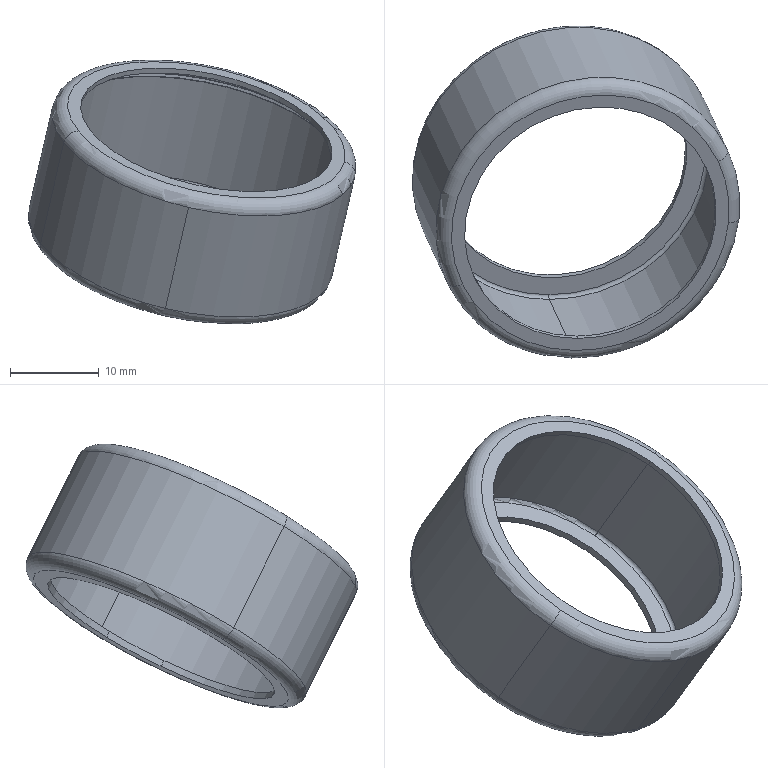Part | SolidWorks | features BaseBody 1 | 1 solid | 40 faces | box 36.983 x 37.484 x 29.782 mm | volume 1472 mm3 | torus 17 | cylinder 15 | plane 4 | cone 3 | spline 1 | commonest cylinder face diameters 28.5 x3 29 x3 33.55 x3 33.75 x3 35.02 x3
STEP:
#1=CARTESIAN_POINT('',(1955.93,-190.672,883.399));
#2=VERTEX_POINT('',#1);
#3=CARTESIAN_POINT('',(1954.896,-184.524,886.692));
#4=VERTEX_POINT('',#3);
#5=CARTESIAN_POINT('',(1942.041,-190.672,886.589));
#6=DIRECTION('',(0.2015,-0.436,0.8771));
#7=DIRECTION('',(-0.9021,-0.4315,-0.007269));
#8=AXIS2_PLACEMENT_3D('',#5,#6,#7);
#9=CIRCLE('',#8,14.25);
#10=EDGE_CURVE('',#2,#4,#9,.T.);
#11=ORIENTED_EDGE('',*,*,#10,.F.);
#12=CARTESIAN_POINT('',(1956.081,-190.999,884.056));
#13=VERTEX_POINT('',#12);
#14=CARTESIAN_POINT('',(1955.918,-190.646,883.346));
#15=DIRECTION('',(0.2015,-0.436,0.8771));
#16=VECTOR('',#15,1000.);
#17=LINE('',#14,#16);
#18=EDGE_CURVE('',#2,#13,#17,.T.);
#19=ORIENTED_EDGE('',*,*,#18,.T.);
#20=CARTESIAN_POINT('',(1955.047,-184.851,887.35));
#21=VERTEX_POINT('',#20);
#22=CARTESIAN_POINT('',(1942.192,-190.999,887.247));
#23=DIRECTION('',(-0.2015,0.436,-0.8771));
#24=DIRECTION('',(0.9021,0.4315,0.007269));
#25=AXIS2_PLACEMENT_3D('',#22,#23,#24);
#26=CIRCLE('',#25,14.25);
#27=EDGE_CURVE('',#21,#13,#26,.T.);
#28=ORIENTED_EDGE('',*,*,#27,.F.);
#29=CARTESIAN_POINT('',(1955.047,-184.851,887.35));
#30=DIRECTION('',(0.2015,-0.436,0.8771));
#31=VECTOR('',#30,1000.);
#32=LINE('',#29,#31);
#33=EDGE_CURVE('',#4,#21,#32,.T.);
#34=ORIENTED_EDGE('',*,*,#33,.F.);
#35=EDGE_LOOP('',(#11,#19,#28,#34));
#36=FACE_OUTER_BOUND('',#35,.T.);
#37=CARTESIAN_POINT('',(1942.029,-190.646,886.536));
#38=DIRECTION('',(0.2015,-0.436,0.8771));
#39=DIRECTION('',(0.9746,0.,-0.2239));
#40=AXIS2_PLACEMENT_3D('',#37,#38,#39);
#41=CYLINDRICAL_SURFACE('',#40,14.25);
#42=ADVANCED_FACE('',(#36),#41,.F.);
#43=CARTESIAN_POINT('',(1957.645,-190.672,883.005));
#44=VERTEX_POINT('',#43);
#45=CARTESIAN_POINT('',(1927.599,-197.58,886.472));
#46=VERTEX_POINT('',#45);
#47=CARTESIAN_POINT('',(1942.041,-190.672,886.589));
#48=DIRECTION('',(-0.2015,0.436,-0.8771));
#49=DIRECTION('',(0.9021,0.4315,0.007269));
#50=AXIS2_PLACEMENT_3D('',#47,#48,#49);
#51=CIRCLE('',#50,16.01);
#52=EDGE_CURVE('',#44,#46,#51,.T.);
#53=ORIENTED_EDGE('',*,*,#52,.F.);
#54=CARTESIAN_POINT('',(1959.409,-191.326,883.984));
#55=VERTEX_POINT('',#54);
#56=CARTESIAN_POINT('',(1957.947,-191.326,884.32));
#57=DIRECTION('',(-0.09761,-0.8999,-0.425));
#58=DIRECTION('',(0.,0.427,-0.9043));
#59=AXIS2_PLACEMENT_3D('',#56,#57,#58);
#60=CIRCLE('',#59,1.5);
#61=EDGE_CURVE('',#44,#55,#60,.T.);
#62=ORIENTED_EDGE('',*,*,#61,.T.);
#63=CARTESIAN_POINT('',(1940.634,-207.084,880.464));
#64=VERTEX_POINT('',#63);
#65=CARTESIAN_POINT('',(1942.344,-191.326,887.904));
#66=DIRECTION('',(-0.2015,0.436,-0.8771));
#67=DIRECTION('',(0.9021,0.4315,0.007269));
#68=AXIS2_PLACEMENT_3D('',#65,#66,#67);
#69=CIRCLE('',#68,17.51);
#70=EDGE_CURVE('',#55,#64,#69,.T.);
#71=ORIENTED_EDGE('',*,*,#70,.T.);
#72=CARTESIAN_POINT('',(1926.548,-198.881,887.777));
#73=VERTEX_POINT('',#72);
#74=CARTESIAN_POINT('',(1942.344,-191.326,887.904));
#75=DIRECTION('',(-0.2015,0.436,-0.8771));
#76=DIRECTION('',(0.9021,0.4315,0.007269));
#77=AXIS2_PLACEMENT_3D('',#74,#75,#76);
#78=CIRCLE('',#77,17.51);
#79=EDGE_CURVE('',#64,#73,#78,.T.);
#80=ORIENTED_EDGE('',*,*,#79,.T.);
#81=CARTESIAN_POINT('',(1927.901,-198.234,887.788));
#82=DIRECTION('',(-0.3816,0.7898,0.4803));
#83=DIRECTION('',(-0.2015,0.436,-0.8771));
#84=AXIS2_PLACEMENT_3D('',#81,#82,#83);
#85=CIRCLE('',#84,1.5);
#86=EDGE_CURVE('',#46,#73,#85,.T.);
#87=ORIENTED_EDGE('',*,*,#86,.F.);
#88=EDGE_LOOP('',(#53,#62,#71,#80,#87));
#89=FACE_OUTER_BOUND('',#88,.T.);
#90=CARTESIAN_POINT('',(1942.344,-191.326,887.904));
#91=DIRECTION('',(0.2015,-0.436,0.8771));
#92=DIRECTION('',(0.9746,0.,-0.2239));
#93=AXIS2_PLACEMENT_3D('',#90,#91,#92);
#94=TOROIDAL_SURFACE('',#93,16.01,1.5);
#95=ADVANCED_FACE('',(#89),#94,.T.);
#96=ORIENTED_EDGE('',*,*,#79,.F.);
#97=CARTESIAN_POINT('',(1943.253,-212.752,891.866));
#98=VERTEX_POINT('',#97);
#99=CARTESIAN_POINT('',(1940.582,-206.971,880.235));
#100=DIRECTION('',(0.2015,-0.436,0.8771));
#101=VECTOR('',#100,1000.);
#102=LINE('',#99,#101);
#103=EDGE_CURVE('',#64,#98,#102,.T.);
#104=ORIENTED_EDGE('',*,*,#103,.T.);
#105=CARTESIAN_POINT('',(1929.167,-204.549,899.179));
#106=VERTEX_POINT('',#105);
#107=CARTESIAN_POINT('',(1944.963,-196.994,899.307));
#108=DIRECTION('',(0.2015,-0.436,0.8771));
#109=DIRECTION('',(0.9726,0.195,-0.1265));
#110=AXIS2_PLACEMENT_3D('',#107,#108,#109);
#111=CIRCLE('',#110,17.51);
#112=EDGE_CURVE('',#106,#98,#111,.T.);
#113=ORIENTED_EDGE('',*,*,#112,.F.);
#114=CARTESIAN_POINT('',(1926.548,-198.881,887.777));
#115=DIRECTION('',(-0.2015,0.436,-0.8771));
#116=VECTOR('',#115,1000.);
#117=LINE('',#114,#116);
#118=EDGE_CURVE('',#106,#73,#117,.T.);
#119=ORIENTED_EDGE('',*,*,#118,.T.);
#120=EDGE_LOOP('',(#96,#104,#113,#119));
#121=FACE_OUTER_BOUND('',#120,.T.);
#122=CARTESIAN_POINT('',(1942.291,-191.213,887.676));
#123=DIRECTION('',(0.2015,-0.436,0.8771));
#124=DIRECTION('',(-0.09761,-0.8999,-0.425));
#125=AXIS2_PLACEMENT_3D('',#122,#123,#124);
#126=CYLINDRICAL_SURFACE('',#125,17.51);
#127=ADVANCED_FACE('',(#121),#126,.T.);
#128=ORIENTED_EDGE('',*,*,#112,.T.);
#129=CARTESIAN_POINT('',(1962.028,-196.994,895.387));
#130=VERTEX_POINT('',#129);
#131=CARTESIAN_POINT('',(1944.963,-196.994,899.307));
#132=DIRECTION('',(0.2015,-0.436,0.8771));
#133=DIRECTION('',(0.9726,0.195,-0.1265));
#134=AXIS2_PLACEMENT_3D('',#131,#132,#133);
#135=CIRCLE('',#134,17.51);
#136=EDGE_CURVE('',#98,#130,#135,.T.);
#137=ORIENTED_EDGE('',*,*,#136,.T.);
#138=CARTESIAN_POINT('',(1960.868,-197.648,897.038));
#139=VERTEX_POINT('',#138);
#140=CARTESIAN_POINT('',(1960.566,-196.994,895.723));
#141=DIRECTION('',(-0.09761,-0.8999,-0.425));
#142=DIRECTION('',(0.,0.427,-0.9043));
#143=AXIS2_PLACEMENT_3D('',#140,#141,#142);
#144=CIRCLE('',#143,1.5);
#145=EDGE_CURVE('',#130,#139,#144,.T.);
#146=ORIENTED_EDGE('',*,*,#145,.T.);
#147=CARTESIAN_POINT('',(1930.822,-204.556,900.506));
#148=VERTEX_POINT('',#147);
#149=CARTESIAN_POINT('',(1945.265,-197.648,900.622));
#150=DIRECTION('',(-0.2015,0.436,-0.8771));
#151=DIRECTION('',(0.9021,0.4315,0.007269));
#152=AXIS2_PLACEMENT_3D('',#149,#150,#151);
#153=CIRCLE('',#152,16.01);
#154=EDGE_CURVE('',#139,#148,#153,.T.);
#155=ORIENTED_EDGE('',*,*,#154,.T.);
#156=CARTESIAN_POINT('',(1930.52,-203.902,899.19));
#157=DIRECTION('',(0.3816,-0.7898,-0.4803));
#158=DIRECTION('',(-0.9021,-0.4315,-0.007269));
#159=AXIS2_PLACEMENT_3D('',#156,#157,#158);
#160=CIRCLE('',#159,1.5);
#161=EDGE_CURVE('',#148,#106,#160,.T.);
#162=ORIENTED_EDGE('',*,*,#161,.T.);
#163=EDGE_LOOP('',(#128,#137,#146,#155,#162));
#164=FACE_OUTER_BOUND('',#163,.T.);
#165=CARTESIAN_POINT('',(1944.963,-196.994,899.307));
#166=DIRECTION('',(0.2015,-0.436,0.8771));
#167=DIRECTION('',(0.9746,0.,-0.2239));
#168=AXIS2_PLACEMENT_3D('',#165,#166,#167);
#169=TOROIDAL_SURFACE('',#168,16.01,1.5);
#170=ADVANCED_FACE('',(#164),#169,.T.);
#171=CARTESIAN_POINT('',(1943.729,-210.436,893.934));
#172=VERTEX_POINT('',#171);
#173=CARTESIAN_POINT('',(1958.224,-191.131,900.201));
#174=VERTEX_POINT('',#173);
#175=CARTESIAN_POINT('',(1945.144,-197.387,900.096));
#176=DIRECTION('',(0.2015,-0.436,0.8771));
#177=DIRECTION('',(-0.9021,-0.4315,-0.007269));
#178=AXIS2_PLACEMENT_3D('',#175,#176,#177);
#179=CIRCLE('',#178,14.5);
#180=EDGE_CURVE('',#172,#174,#179,.T.);
#181=ORIENTED_EDGE('',*,*,#180,.F.);
#182=CARTESIAN_POINT('',(1943.849,-210.697,894.461));
#183=VERTEX_POINT('',#182);
#184=CARTESIAN_POINT('',(1943.716,-210.41,893.882));
#185=DIRECTION('',(0.2015,-0.436,0.8771));
#186=VECTOR('',#185,1000.);
#187=LINE('',#184,#186);
#188=EDGE_CURVE('',#172,#183,#187,.T.);
#189=ORIENTED_EDGE('',*,*,#188,.T.);
#190=CARTESIAN_POINT('',(1958.345,-191.392,900.728));
#191=VERTEX_POINT('',#190);
#192=CARTESIAN_POINT('',(1945.265,-197.648,900.622));
#193=DIRECTION('',(-0.2015,0.436,-0.8771));
#194=DIRECTION('',(0.9021,0.4315,0.007269));
#195=AXIS2_PLACEMENT_3D('',#192,#193,#194);
#196=CIRCLE('',#195,14.5);
#197=EDGE_CURVE('',#191,#183,#196,.T.);
#198=ORIENTED_EDGE('',*,*,#197,.F.);
#199=CARTESIAN_POINT('',(1958.345,-191.392,900.728));
#200=DIRECTION('',(0.2015,-0.436,0.8771));
#201=VECTOR('',#200,1000.);
#202=LINE('',#199,#201);
#203=EDGE_CURVE('',#174,#191,#202,.T.);
#204=ORIENTED_EDGE('',*,*,#203,.F.);
#205=EDGE_LOOP('',(#181,#189,#198,#204));
#206=FACE_OUTER_BOUND('',#205,.T.);
#207=CARTESIAN_POINT('',(1945.132,-197.36,900.043));
#208=DIRECTION('',(0.2015,-0.436,0.8771));
#209=DIRECTION('',(-0.09761,-0.8999,-0.425));
#210=AXIS2_PLACEMENT_3D('',#207,#208,#209);
#211=CYLINDRICAL_SURFACE('',#210,14.5);
#212=ADVANCED_FACE('',(#206),#211,.F.);
#213=CARTESIAN_POINT('',(1960.286,-189.931,899.868));
#214=VERTEX_POINT('',#213);
#215=CARTESIAN_POINT('',(1943.416,-212.399,892.574));
#216=VERTEX_POINT('',#215);
#217=CARTESIAN_POINT('',(1945.063,-197.212,899.745));
#218=DIRECTION('',(-0.2015,0.436,-0.8771));
#219=DIRECTION('',(0.9021,0.4315,0.007269));
#220=AXIS2_PLACEMENT_3D('',#217,#218,#219);
#221=CIRCLE('',#220,16.875);
#222=EDGE_CURVE('',#214,#216,#221,.T.);
#223=ORIENTED_EDGE('',*,*,#222,.T.);
#224=CARTESIAN_POINT('',(1943.536,-212.213,893.095));
#225=VERTEX_POINT('',#224);
#226=CARTESIAN_POINT('',(1943.455,-212.039,892.744));
#227=DIRECTION('',(-0.9746,0.,0.2239));
#228=DIRECTION('',(0.2239,0.,0.9746));
#229=AXIS2_PLACEMENT_3D('',#226,#227,#228);
#230=CIRCLE('',#229,0.4);
#231=EDGE_CURVE('',#216,#225,#230,.T.);
#232=ORIENTED_EDGE('',*,*,#231,.T.);
#233=CARTESIAN_POINT('',(1960.006,-190.278,900.216));
#234=VERTEX_POINT('',#233);
#235=CARTESIAN_POINT('',(1945.144,-197.387,900.096));
#236=DIRECTION('',(-0.2015,0.436,-0.8771));
#237=DIRECTION('',(0.9021,0.4315,0.007269));
#238=AXIS2_PLACEMENT_3D('',#235,#236,#237);
#239=CIRCLE('',#238,16.475);
#240=EDGE_CURVE('',#234,#225,#239,.T.);
#241=ORIENTED_EDGE('',*,*,#240,.F.);
#242=CARTESIAN_POINT('',(1959.926,-190.104,899.865));
#243=DIRECTION('',(-0.3816,0.7898,0.4803));
#244=DIRECTION('',(0.2015,-0.436,0.8771));
#245=AXIS2_PLACEMENT_3D('',#242,#243,#244);
#246=CIRCLE('',#245,0.4);
#247=EDGE_CURVE('',#234,#214,#246,.T.);
#248=ORIENTED_EDGE('',*,*,#247,.T.);
#249=EDGE_LOOP('',(#223,#232,#241,#248));
#250=FACE_OUTER_BOUND('',#249,.T.);
#251=CARTESIAN_POINT('',(1945.063,-197.212,899.745));
#252=DIRECTION('',(0.2015,-0.436,0.8771));
#253=DIRECTION('',(-0.09761,-0.8999,-0.425));
#254=AXIS2_PLACEMENT_3D('',#251,#252,#253);
#255=TOROIDAL_SURFACE('',#254,16.475,0.4);
#256=ADVANCED_FACE('',(#250),#255,.F.);
#257=CARTESIAN_POINT('',(1943.235,-212.006,891.784));
#258=VERTEX_POINT('',#257);
#259=CARTESIAN_POINT('',(1960.105,-189.539,899.078));
#260=VERTEX_POINT('',#259);
#261=CARTESIAN_POINT('',(1944.882,-196.82,898.955));
#262=DIRECTION('',(0.2015,-0.436,0.8771));
#263=DIRECTION('',(-0.9021,-0.4315,-0.007269));
#264=AXIS2_PLACEMENT_3D('',#261,#262,#263);
#265=CIRCLE('',#264,16.875);
#266=EDGE_CURVE('',#258,#260,#265,.T.);
#267=ORIENTED_EDGE('',*,*,#266,.F.);
#268=CARTESIAN_POINT('',(1943.223,-211.98,891.732));
#269=DIRECTION('',(0.2015,-0.436,0.8771));
#270=VECTOR('',#269,1000.);
#271=LINE('',#268,#270);
#272=EDGE_CURVE('',#258,#216,#271,.T.);
#273=ORIENTED_EDGE('',*,*,#272,.T.);
#274=ORIENTED_EDGE('',*,*,#222,.F.);
#275=CARTESIAN_POINT('',(1960.286,-189.931,899.868));
#276=DIRECTION('',(0.2015,-0.436,0.8771));
#277=VECTOR('',#276,1000.);
#278=LINE('',#275,#277);
#279=EDGE_CURVE('',#260,#214,#278,.T.);
#280=ORIENTED_EDGE('',*,*,#279,.F.);
#281=EDGE_LOOP('',(#267,#273,#274,#280));
#282=FACE_OUTER_BOUND('',#281,.T.);
#283=CARTESIAN_POINT('',(1944.87,-196.793,898.903));
#284=DIRECTION('',(0.2015,-0.436,0.8771));
#285=DIRECTION('',(-0.09761,-0.8999,-0.425));
#286=AXIS2_PLACEMENT_3D('',#283,#284,#285);
#287=CYLINDRICAL_SURFACE('',#286,16.875);
#288=ADVANCED_FACE('',(#282),#287,.F.);
#289=CARTESIAN_POINT('',(1960.088,-189.519,899.033));
#290=VERTEX_POINT('',#289);
#291=CARTESIAN_POINT('',(1943.225,-211.977,891.742));
#292=VERTEX_POINT('',#291);
#293=CARTESIAN_POINT('',(1944.871,-196.797,898.91));
#294=DIRECTION('',(-0.2015,0.436,-0.8771));
#295=DIRECTION('',(0.9021,0.4315,0.007269));
#296=AXIS2_PLACEMENT_3D('',#293,#294,#295);
#297=CIRCLE('',#296,16.868);
#298=EDGE_CURVE('',#290,#292,#297,.T.);
#299=ORIENTED_EDGE('',*,*,#298,.T.);
#300=CARTESIAN_POINT('',(1943.254,-211.826,891.869));
#301=DIRECTION('',(-0.9746,0.,0.2239));
#302=DIRECTION('',(0.2239,0.,0.9746));
#303=AXIS2_PLACEMENT_3D('',#300,#301,#302);
#304=CIRCLE('',#303,0.2);
#305=EDGE_CURVE('',#292,#258,#304,.T.);
#306=ORIENTED_EDGE('',*,*,#305,.T.);
#307=ORIENTED_EDGE('',*,*,#266,.T.);
#308=CARTESIAN_POINT('',(1959.925,-189.625,899.077));
#309=DIRECTION('',(-0.3816,0.7898,0.4803));
#310=DIRECTION('',(0.9021,0.4315,0.007269));
#311=AXIS2_PLACEMENT_3D('',#308,#309,#310);
#312=CIRCLE('',#311,0.2);
#313=EDGE_CURVE('',#260,#290,#312,.T.);
#314=ORIENTED_EDGE('',*,*,#313,.T.);
#315=EDGE_LOOP('',(#299,#306,#307,#314));
#316=FACE_OUTER_BOUND('',#315,.T.);
#317=CARTESIAN_POINT('',(1944.882,-196.82,898.955));
#318=DIRECTION('',(0.2015,-0.436,0.8771));
#319=DIRECTION('',(-0.09761,-0.8999,-0.425));
#320=AXIS2_PLACEMENT_3D('',#317,#318,#319);
#321=TOROIDAL_SURFACE('',#320,16.675,0.2);
#322=ADVANCED_FACE('',(#316),#321,.F.);
#323=CARTESIAN_POINT('',(1943.168,-211.759,891.496));
#324=VERTEX_POINT('',#323);
#325=CARTESIAN_POINT('',(1959.946,-189.416,898.749));
#326=VERTEX_POINT('',#325);
#327=CARTESIAN_POINT('',(1944.807,-196.656,898.627));
#328=DIRECTION('',(0.2015,-0.436,0.8771));
#329=DIRECTION('',(-0.9021,-0.4315,-0.007269));
#330=AXIS2_PLACEMENT_3D('',#327,#328,#329);
#331=CIRCLE('',#330,16.782);
#332=EDGE_CURVE('',#324,#326,#331,.T.);
#333=ORIENTED_EDGE('',*,*,#332,.F.);
#334=CARTESIAN_POINT('',(1943.158,-211.72,891.452));
#335=DIRECTION('',(0.1693,-0.6541,0.7372));
#336=VECTOR('',#335,1000.);
#337=LINE('',#334,#336);
#338=EDGE_CURVE('',#324,#292,#337,.T.);
#339=ORIENTED_EDGE('',*,*,#338,.T.);
#340=ORIENTED_EDGE('',*,*,#298,.F.);
#341=CARTESIAN_POINT('',(1960.088,-189.519,899.033));
#342=DIRECTION('',(0.4281,-0.3095,0.8491));
#343=VECTOR('',#342,1000.);
#344=LINE('',#341,#343);
#345=EDGE_CURVE('',#326,#290,#344,.T.);
#346=ORIENTED_EDGE('',*,*,#345,.F.);
#347=EDGE_LOOP('',(#333,#339,#340,#346));
#348=FACE_OUTER_BOUND('',#347,.T.);
#349=CARTESIAN_POINT('',(1944.795,-196.631,898.576));
#350=DIRECTION('',(0.2015,-0.436,0.8771));
#351=DIRECTION('',(-0.09761,-0.8999,-0.425));
#352=AXIS2_PLACEMENT_3D('',#349,#350,#351);
#353=CONICAL_SURFACE('',#352,16.766,0.2618);
#354=ADVANCED_FACE('',(#348),#353,.F.);
#355=CARTESIAN_POINT('',(1929.668,-203.897,898.505));
#356=VERTEX_POINT('',#355);
#357=CARTESIAN_POINT('',(1944.807,-196.656,898.627));
#358=DIRECTION('',(0.2015,-0.436,0.8771));
#359=DIRECTION('',(-0.9021,-0.4315,-0.007269));
#360=AXIS2_PLACEMENT_3D('',#357,#358,#359);
#361=CIRCLE('',#360,16.782);
#362=EDGE_CURVE('',#356,#324,#361,.T.);
#363=ORIENTED_EDGE('',*,*,#362,.T.);
#364=CARTESIAN_POINT('',(1943.159,-211.73,891.453));
#365=VERTEX_POINT('',#364);
#366=CARTESIAN_POINT('',(1943.139,-211.91,891.368));
#367=DIRECTION('',(-0.9746,0.,0.2239));
#368=DIRECTION('',(0.2239,0.,0.9746));
#369=AXIS2_PLACEMENT_3D('',#366,#367,#368);
#370=CIRCLE('',#369,0.2);
#371=EDGE_CURVE('',#324,#365,#370,.T.);
#372=ORIENTED_EDGE('',*,*,#371,.T.);
#373=CARTESIAN_POINT('',(1929.663,-203.872,898.46));
#374=VERTEX_POINT('',#373);
#375=CARTESIAN_POINT('',(1944.796,-196.634,898.582));
#376=DIRECTION('',(-0.2015,0.436,-0.8771));
#377=DIRECTION('',(0.9021,0.4315,0.007269));
#378=AXIS2_PLACEMENT_3D('',#375,#376,#377);
#379=CIRCLE('',#378,16.775);
#380=EDGE_CURVE('',#365,#374,#379,.T.);
#381=ORIENTED_EDGE('',*,*,#380,.T.);
#382=CARTESIAN_POINT('',(1929.483,-203.958,898.458));
#383=DIRECTION('',(0.3816,-0.7898,-0.4803));
#384=DIRECTION('',(0.9235,0.3039,0.234));
#385=AXIS2_PLACEMENT_3D('',#382,#383,#384);
#386=CIRCLE('',#385,0.2);
#387=EDGE_CURVE('',#374,#356,#386,.T.);
#388=ORIENTED_EDGE('',*,*,#387,.T.);
#389=EDGE_LOOP('',(#363,#372,#381,#388));
#390=FACE_OUTER_BOUND('',#389,.T.);
#391=CARTESIAN_POINT('',(1944.796,-196.634,898.582));
#392=DIRECTION('',(0.2015,-0.436,0.8771));
#393=DIRECTION('',(-0.09761,-0.8999,-0.425));
#394=AXIS2_PLACEMENT_3D('',#391,#392,#393);
#395=TOROIDAL_SURFACE('',#394,16.975,0.2);
#396=ADVANCED_FACE('',(#390),#395,.T.);
#397=CARTESIAN_POINT('',(1940.636,-206.27,880.469));
#398=VERTEX_POINT('',#397);
#399=CARTESIAN_POINT('',(1957.406,-183.936,887.719));
#400=VERTEX_POINT('',#399);
#401=CARTESIAN_POINT('',(1942.273,-191.173,887.597));
#402=DIRECTION('',(0.2015,-0.436,0.8771));
#403=DIRECTION('',(-0.9021,-0.4315,-0.007269));
#404=AXIS2_PLACEMENT_3D('',#401,#402,#403);
#405=CIRCLE('',#404,16.775);
#406=EDGE_CURVE('',#398,#400,#405,.T.);
#407=ORIENTED_EDGE('',*,*,#406,.F.);
#408=CARTESIAN_POINT('',(1940.585,-206.161,880.249));
#409=DIRECTION('',(0.2015,-0.436,0.8771));
#410=VECTOR('',#409,1000.);
#411=LINE('',#408,#410);
#412=EDGE_CURVE('',#398,#365,#411,.T.);
#413=ORIENTED_EDGE('',*,*,#412,.T.);
#414=CARTESIAN_POINT('',(1959.929,-189.396,898.704));
#415=VERTEX_POINT('',#414);
#416=CARTESIAN_POINT('',(1944.796,-196.634,898.582));
#417=DIRECTION('',(-0.2015,0.436,-0.8771));
#418=DIRECTION('',(0.9021,0.4315,0.007269));
#419=AXIS2_PLACEMENT_3D('',#416,#417,#418);
#420=CIRCLE('',#419,16.775);
#421=EDGE_CURVE('',#415,#365,#420,.T.);
#422=ORIENTED_EDGE('',*,*,#421,.F.);
#423=CARTESIAN_POINT('',(1959.929,-189.396,898.704));
#424=DIRECTION('',(-0.2015,0.436,-0.8771));
#425=VECTOR('',#424,1000.);
#426=LINE('',#423,#425);
#427=EDGE_CURVE('',#415,#400,#426,.T.);
#428=ORIENTED_EDGE('',*,*,#427,.T.);
#429=EDGE_LOOP('',(#407,#413,#422,#428));
#430=FACE_OUTER_BOUND('',#429,.T.);
#431=CARTESIAN_POINT('',(1942.223,-191.064,887.378));
#432=DIRECTION('',(0.2015,-0.436,0.8771));
#433=DIRECTION('',(-0.09761,-0.8999,-0.425));
#434=AXIS2_PLACEMENT_3D('',#431,#432,#433);
#435=CYLINDRICAL_SURFACE('',#434,16.775);
#436=ADVANCED_FACE('',(#430),#435,.F.);
#437=CARTESIAN_POINT('',(1940.594,-205.735,880.288));
#438=VERTEX_POINT('',#437);
#439=CARTESIAN_POINT('',(1956.964,-183.934,887.366));
#440=VERTEX_POINT('',#439);
#441=CARTESIAN_POINT('',(1942.192,-190.999,887.247));
#442=DIRECTION('',(0.2015,-0.436,0.8771));
#443=DIRECTION('',(-0.9021,-0.4315,-0.007269));
#444=AXIS2_PLACEMENT_3D('',#441,#442,#443);
#445=CIRCLE('',#444,16.375);
#446=EDGE_CURVE('',#438,#440,#445,.T.);
#447=ORIENTED_EDGE('',*,*,#446,.F.);
#448=CARTESIAN_POINT('',(1940.675,-205.91,880.639));
#449=DIRECTION('',(-0.9746,0.,0.2239));
#450=DIRECTION('',(0.2239,0.,0.9746));
#451=AXIS2_PLACEMENT_3D('',#448,#449,#450);
#452=CIRCLE('',#451,0.4);
#453=EDGE_CURVE('',#438,#398,#452,.T.);
#454=ORIENTED_EDGE('',*,*,#453,.T.);
#455=ORIENTED_EDGE('',*,*,#406,.T.);
#456=CARTESIAN_POINT('',(1957.045,-184.108,887.716));
#457=DIRECTION('',(-0.3816,0.7898,0.4803));
#458=DIRECTION('',(0.9021,0.4315,0.007269));
#459=AXIS2_PLACEMENT_3D('',#456,#457,#458);
#460=CIRCLE('',#459,0.4);
#461=EDGE_CURVE('',#400,#440,#460,.T.);
#462=ORIENTED_EDGE('',*,*,#461,.T.);
#463=EDGE_LOOP('',(#447,#454,#455,#462));
#464=FACE_OUTER_BOUND('',#463,.T.);
#465=CARTESIAN_POINT('',(1942.273,-191.173,887.597));
#466=DIRECTION('',(0.2015,-0.436,0.8771));
#467=DIRECTION('',(-0.09761,-0.8999,-0.425));
#468=AXIS2_PLACEMENT_3D('',#465,#466,#467);
#469=TOROIDAL_SURFACE('',#468,16.375,0.4);
#470=ADVANCED_FACE('',(#464),#469,.F.);
#471=ORIENTED_EDGE('',*,*,#345,.T.);
#472=CARTESIAN_POINT('',(1929.655,-204.075,898.787));
#473=VERTEX_POINT('',#472);
#474=CARTESIAN_POINT('',(1944.871,-196.797,898.91));
#475=DIRECTION('',(-0.2015,0.436,-0.8771));
#476=DIRECTION('',(-0.9021,-0.4315,-0.007269));
#477=AXIS2_PLACEMENT_3D('',#474,#475,#476);
#478=CIRCLE('',#477,16.868);
#479=EDGE_CURVE('',#473,#290,#478,.T.);
#480=ORIENTED_EDGE('',*,*,#479,.F.);
#481=CARTESIAN_POINT('',(1929.655,-204.075,898.787));
#482=DIRECTION('',(0.03888,0.5328,-0.8453));
#483=VECTOR('',#482,1000.);
#484=LINE('',#481,#483);
#485=EDGE_CURVE('',#473,#356,#484,.T.);
#486=ORIENTED_EDGE('',*,*,#485,.T.);
#487=CARTESIAN_POINT('',(1944.807,-196.656,898.627));
#488=DIRECTION('',(0.2015,-0.436,0.8771));
#489=DIRECTION('',(0.9021,0.4315,0.007269));
#490=AXIS2_PLACEMENT_3D('',#487,#488,#489);
#491=CIRCLE('',#490,16.782);
#492=EDGE_CURVE('',#326,#356,#491,.T.);
#493=ORIENTED_EDGE('',*,*,#492,.F.);
#494=EDGE_LOOP('',(#471,#480,#486,#493));
#495=FACE_OUTER_BOUND('',#494,.T.);
#496=CARTESIAN_POINT('',(1944.795,-196.631,898.576));
#497=DIRECTION('',(0.2015,-0.436,0.8771));
#498=DIRECTION('',(-0.09761,-0.8999,-0.425));
#499=AXIS2_PLACEMENT_3D('',#496,#497,#498);
#500=CONICAL_SURFACE('',#499,16.766,0.2618);
#501=ADVANCED_FACE('',(#495),#500,.F.);
#502=CARTESIAN_POINT('',(1960.109,-189.31,898.705));
#503=DIRECTION('',(0.3816,-0.7898,-0.4803));
#504=DIRECTION('',(-0.8192,-0.5296,0.22));
#505=AXIS2_PLACEMENT_3D('',#502,#503,#504);
#506=CIRCLE('',#505,0.2);
#507=EDGE_CURVE('',#326,#415,#506,.T.);
#508=ORIENTED_EDGE('',*,*,#507,.F.);
#509=ORIENTED_EDGE('',*,*,#492,.T.);
#510=ORIENTED_EDGE('',*,*,#387,.F.);
#511=CARTESIAN_POINT('',(1944.796,-196.634,898.582));
#512=DIRECTION('',(-0.2015,0.436,-0.8771));
#513=DIRECTION('',(-0.9021,-0.4315,-0.007269));
#514=AXIS2_PLACEMENT_3D('',#511,#512,#513);
#515=CIRCLE('',#514,16.775);
#516=EDGE_CURVE('',#374,#415,#515,.T.);
#517=ORIENTED_EDGE('',*,*,#516,.T.);
#518=EDGE_LOOP('',(#508,#509,#510,#517));
#519=FACE_OUTER_BOUND('',#518,.T.);
#520=CARTESIAN_POINT('',(1944.796,-196.634,898.582));
#521=DIRECTION('',(0.2015,-0.436,0.8771));
#522=DIRECTION('',(-0.09761,-0.8999,-0.425));
#523=AXIS2_PLACEMENT_3D('',#520,#521,#522);
#524=TOROIDAL_SURFACE('',#523,16.975,0.2);
#525=ADVANCED_FACE('',(#519),#524,.T.);
#526=ORIENTED_EDGE('',*,*,#427,.F.);
#527=ORIENTED_EDGE('',*,*,#516,.F.);
#528=CARTESIAN_POINT('',(1927.14,-198.411,887.475));
#529=VERTEX_POINT('',#528);
#530=CARTESIAN_POINT('',(1929.663,-203.872,898.46));
#531=DIRECTION('',(0.2015,-0.436,0.8771));
#532=VECTOR('',#531,1000.);
#533=LINE('',#530,#532);
#534=EDGE_CURVE('',#529,#374,#533,.T.);
#535=ORIENTED_EDGE('',*,*,#534,.F.);
#536=CARTESIAN_POINT('',(1942.273,-191.173,887.597));
#537=DIRECTION('',(0.2015,-0.436,0.8771));
#538=DIRECTION('',(0.9021,0.4315,0.007269));
#539=AXIS2_PLACEMENT_3D('',#536,#537,#538);
#540=CIRCLE('',#539,16.775);
#541=EDGE_CURVE('',#400,#529,#540,.T.);
#542=ORIENTED_EDGE('',*,*,#541,.F.);
#543=EDGE_LOOP('',(#526,#527,#535,#542));
#544=FACE_OUTER_BOUND('',#543,.T.);
#545=CARTESIAN_POINT('',(1942.223,-191.064,887.378));
#546=DIRECTION('',(0.2015,-0.436,0.8771));
#547=DIRECTION('',(-0.09761,-0.8999,-0.425));
#548=AXIS2_PLACEMENT_3D('',#545,#546,#547);
#549=CYLINDRICAL_SURFACE('',#548,16.775);
#550=ADVANCED_FACE('',(#544),#549,.F.);
#551=ORIENTED_EDGE('',*,*,#461,.F.);
#552=ORIENTED_EDGE('',*,*,#541,.T.);
#553=CARTESIAN_POINT('',(1927.42,-198.064,887.128));
#554=VERTEX_POINT('',#553);
#555=CARTESIAN_POINT('',(1927.501,-198.238,887.478));
#556=DIRECTION('',(-0.3816,0.7898,0.4803));
#557=DIRECTION('',(-0.9021,-0.4315,-0.007269));
#558=AXIS2_PLACEMENT_3D('',#555,#556,#557);
#559=CIRCLE('',#558,0.4);
#560=EDGE_CURVE('',#554,#529,#559,.T.);
#561=ORIENTED_EDGE('',*,*,#560,.F.);
#562=CARTESIAN_POINT('',(1942.192,-190.999,887.247));
#563=DIRECTION('',(0.2015,-0.436,0.8771));
#564=DIRECTION('',(0.9021,0.4315,0.007269));
#565=AXIS2_PLACEMENT_3D('',#562,#563,#564);
#566=CIRCLE('',#565,16.375);
#567=EDGE_CURVE('',#440,#554,#566,.T.);
#568=ORIENTED_EDGE('',*,*,#567,.F.);
#569=EDGE_LOOP('',(#551,#552,#561,#568));
#570=FACE_OUTER_BOUND('',#569,.T.);
#571=CARTESIAN_POINT('',(1942.273,-191.173,887.597));
#572=DIRECTION('',(0.2015,-0.436,0.8771));
#573=DIRECTION('',(-0.09761,-0.8999,-0.425));
#574=AXIS2_PLACEMENT_3D('',#571,#572,#573);
#575=TOROIDAL_SURFACE('',#574,16.375,0.4);
#576=ADVANCED_FACE('',(#570),#575,.F.);
#577=CARTESIAN_POINT('',(1942.192,-190.999,887.247));
#578=DIRECTION('',(0.2015,-0.436,0.8771));
#579=DIRECTION('',(-0.9021,-0.4315,-0.007269));
#580=AXIS2_PLACEMENT_3D('',#577,#578,#579);
#581=CIRCLE('',#580,16.375);
#582=EDGE_CURVE('',#554,#438,#581,.T.);
#583=ORIENTED_EDGE('',*,*,#582,.T.);
#584=ORIENTED_EDGE('',*,*,#446,.T.);
#585=ORIENTED_EDGE('',*,*,#567,.T.);
#586=EDGE_LOOP('',(#583,#584,#585));
#587=FACE_OUTER_BOUND('',#586,.T.);
#588=ORIENTED_EDGE('',*,*,#27,.T.);
#589=CARTESIAN_POINT('',(1929.337,-197.147,887.143));
#590=VERTEX_POINT('',#589);
#591=CARTESIAN_POINT('',(1942.192,-190.999,887.247));
#592=DIRECTION('',(-0.2015,0.436,-0.8771));
#593=DIRECTION('',(0.9021,0.4315,0.007269));
#594=AXIS2_PLACEMENT_3D('',#591,#592,#593);
#595=CIRCLE('',#594,14.25);
#596=EDGE_CURVE('',#13,#590,#595,.T.);
#597=ORIENTED_EDGE('',*,*,#596,.T.);
#598=CARTESIAN_POINT('',(1942.192,-190.999,887.247));
#599=DIRECTION('',(-0.2015,0.436,-0.8771));
#600=DIRECTION('',(-0.9021,-0.4315,-0.007269));
#601=AXIS2_PLACEMENT_3D('',#598,#599,#600);
#602=CIRCLE('',#601,14.25);
#603=EDGE_CURVE('',#590,#21,#602,.T.);
#604=ORIENTED_EDGE('',*,*,#603,.T.);
#605=EDGE_LOOP('',(#588,#597,#604));
#606=FACE_BOUND('',#605,.T.);
#607=CARTESIAN_POINT('',(1957.134,-206.325,876.196));
#608=DIRECTION('',(0.2015,-0.436,0.8771));
#609=DIRECTION('',(0.09761,0.8999,0.425));
#610=AXIS2_PLACEMENT_3D('',#607,#608,#609);
#611=PLANE('',#610);
#612=ADVANCED_FACE('',(#587,#606),#611,.T.);
#613=ORIENTED_EDGE('',*,*,#453,.F.);
#614=ORIENTED_EDGE('',*,*,#582,.F.);
#615=ORIENTED_EDGE('',*,*,#560,.T.);
#616=CARTESIAN_POINT('',(1942.273,-191.173,887.597));
#617=DIRECTION('',(0.2015,-0.436,0.8771));
#618=DIRECTION('',(-0.9021,-0.4315,-0.007269));
#619=AXIS2_PLACEMENT_3D('',#616,#617,#618);
#620=CIRCLE('',#619,16.775);
#621=EDGE_CURVE('',#529,#398,#620,.T.);
#622=ORIENTED_EDGE('',*,*,#621,.T.);
#623=EDGE_LOOP('',(#613,#614,#615,#622));
#624=FACE_OUTER_BOUND('',#623,.T.);
#625=CARTESIAN_POINT('',(1942.273,-191.173,887.597));
#626=DIRECTION('',(0.2015,-0.436,0.8771));
#627=DIRECTION('',(-0.09761,-0.8999,-0.425));
#628=AXIS2_PLACEMENT_3D('',#625,#626,#627);
#629=TOROIDAL_SURFACE('',#628,16.375,0.4);
#630=ADVANCED_FACE('',(#624),#629,.F.);
#631=ORIENTED_EDGE('',*,*,#412,.F.);
#632=ORIENTED_EDGE('',*,*,#621,.F.);
#633=ORIENTED_EDGE('',*,*,#534,.T.);
#634=ORIENTED_EDGE('',*,*,#380,.F.);
#635=EDGE_LOOP('',(#631,#632,#633,#634));
#636=FACE_OUTER_BOUND('',#635,.T.);
#637=CARTESIAN_POINT('',(1942.223,-191.064,887.378));
#638=DIRECTION('',(0.2015,-0.436,0.8771));
#639=DIRECTION('',(-0.09761,-0.8999,-0.425));
#640=AXIS2_PLACEMENT_3D('',#637,#638,#639);
#641=CYLINDRICAL_SURFACE('',#640,16.775);
#642=ADVANCED_FACE('',(#636),#641,.F.);
#643=ORIENTED_EDGE('',*,*,#371,.F.);
#644=ORIENTED_EDGE('',*,*,#332,.T.);
#645=ORIENTED_EDGE('',*,*,#507,.T.);
#646=ORIENTED_EDGE('',*,*,#421,.T.);
#647=EDGE_LOOP('',(#643,#644,#645,#646));
#648=FACE_OUTER_BOUND('',#647,.T.);
#649=CARTESIAN_POINT('',(1944.796,-196.634,898.582));
#650=DIRECTION('',(0.2015,-0.436,0.8771));
#651=DIRECTION('',(-0.09761,-0.8999,-0.425));
#652=AXIS2_PLACEMENT_3D('',#649,#650,#651);
#653=TOROIDAL_SURFACE('',#652,16.975,0.2);
#654=ADVANCED_FACE('',(#648),#653,.T.);
#655=ORIENTED_EDGE('',*,*,#338,.F.);
#656=ORIENTED_EDGE('',*,*,#362,.F.);
#657=ORIENTED_EDGE('',*,*,#485,.F.);
#658=CARTESIAN_POINT('',(1944.871,-196.797,898.91));
#659=DIRECTION('',(-0.2015,0.436,-0.8771));
#660=DIRECTION('',(0.9021,0.4315,0.007269));
#661=AXIS2_PLACEMENT_3D('',#658,#659,#660);
#662=CIRCLE('',#661,16.868);
#663=EDGE_CURVE('',#292,#473,#662,.T.);
#664=ORIENTED_EDGE('',*,*,#663,.F.);
#665=EDGE_LOOP('',(#655,#656,#657,#664));
#666=FACE_OUTER_BOUND('',#665,.T.);
#667=CARTESIAN_POINT('',(1944.795,-196.631,898.576));
#668=DIRECTION('',(0.2015,-0.436,0.8771));
#669=DIRECTION('',(-0.09761,-0.8999,-0.425));
#670=AXIS2_PLACEMENT_3D('',#667,#668,#669);
#671=CONICAL_SURFACE('',#670,16.766,0.2618);
#672=ADVANCED_FACE('',(#666),#671,.F.);
#673=ORIENTED_EDGE('',*,*,#305,.F.);
#674=ORIENTED_EDGE('',*,*,#663,.T.);
#675=CARTESIAN_POINT('',(1929.659,-204.1,898.833));
#676=VERTEX_POINT('',#675);
#677=CARTESIAN_POINT('',(1929.839,-204.014,898.834));
#678=DIRECTION('',(-0.3816,0.7898,0.4803));
#679=DIRECTION('',(-0.9021,-0.4315,-0.007269));
#680=AXIS2_PLACEMENT_3D('',#677,#678,#679);
#681=CIRCLE('',#680,0.2);
#682=EDGE_CURVE('',#473,#676,#681,.T.);
#683=ORIENTED_EDGE('',*,*,#682,.T.);
#684=CARTESIAN_POINT('',(1944.882,-196.82,898.955));
#685=DIRECTION('',(0.2015,-0.436,0.8771));
#686=DIRECTION('',(-0.9021,-0.4315,-0.007269));
#687=AXIS2_PLACEMENT_3D('',#684,#685,#686);
#688=CIRCLE('',#687,16.875);
#689=EDGE_CURVE('',#676,#258,#688,.T.);
#690=ORIENTED_EDGE('',*,*,#689,.T.);
#691=EDGE_LOOP('',(#673,#674,#683,#690));
#692=FACE_OUTER_BOUND('',#691,.T.);
#693=CARTESIAN_POINT('',(1944.882,-196.82,898.955));
#694=DIRECTION('',(0.2015,-0.436,0.8771));
#695=DIRECTION('',(-0.09761,-0.8999,-0.425));
#696=AXIS2_PLACEMENT_3D('',#693,#694,#695);
#697=TOROIDAL_SURFACE('',#696,16.675,0.2);
#698=ADVANCED_FACE('',(#692),#697,.F.);
#699=ORIENTED_EDGE('',*,*,#313,.F.);
#700=CARTESIAN_POINT('',(1944.882,-196.82,898.955));
#701=DIRECTION('',(0.2015,-0.436,0.8771));
#702=DIRECTION('',(0.9021,0.4315,0.007269));
#703=AXIS2_PLACEMENT_3D('',#700,#701,#702);
#704=CIRCLE('',#703,16.875);
#705=EDGE_CURVE('',#260,#676,#704,.T.);
#706=ORIENTED_EDGE('',*,*,#705,.T.);
#707=ORIENTED_EDGE('',*,*,#682,.F.);
#708=ORIENTED_EDGE('',*,*,#479,.T.);
#709=EDGE_LOOP('',(#699,#706,#707,#708));
#710=FACE_OUTER_BOUND('',#709,.T.);
#711=CARTESIAN_POINT('',(1960.462,-190.37,898.523));
#712=CARTESIAN_POINT('',(1957.097,-181.906,903.503));
#713=CARTESIAN_POINT('',(1947.799,-178.996,907.086));
#714=CARTESIAN_POINT('',(1938.435,-183.475,907.01));
#715=CARTESIAN_POINT('',(1929.07,-187.954,906.935));
#716=CARTESIAN_POINT('',(1925.547,-196.996,903.249));
#717=CARTESIAN_POINT('',(1930.089,-204.896,898.278));
#718=CARTESIAN_POINT('',(1960.47,-190.376,898.538));
#719=CARTESIAN_POINT('',(1957.104,-181.91,903.52));
#720=CARTESIAN_POINT('',(1947.803,-178.999,907.103));
#721=CARTESIAN_POINT('',(1938.436,-183.479,907.028));
#722=CARTESIAN_POINT('',(1929.069,-187.959,906.952));
#723=CARTESIAN_POINT('',(1925.546,-197.003,903.265));
#724=CARTESIAN_POINT('',(1930.088,-204.906,898.293));
#725=CARTESIAN_POINT('',(1960.476,-190.382,898.554));
#726=CARTESIAN_POINT('',(1957.109,-181.916,903.536));
#727=CARTESIAN_POINT('',(1947.807,-179.004,907.12));
#728=CARTESIAN_POINT('',(1938.439,-183.485,907.045));
#729=CARTESIAN_POINT('',(1929.071,-187.965,906.969));
#730=CARTESIAN_POINT('',(1925.546,-197.011,903.282));
#731=CARTESIAN_POINT('',(1930.09,-204.915,898.309));
#732=CARTESIAN_POINT('',(1960.479,-190.39,898.57));
#733=CARTESIAN_POINT('',(1957.113,-181.924,903.552));
#734=CARTESIAN_POINT('',(1947.811,-179.012,907.136));
#735=CARTESIAN_POINT('',(1938.443,-183.493,907.061));
#736=CARTESIAN_POINT('',(1929.074,-187.973,906.985));
#737=CARTESIAN_POINT('',(1925.55,-197.019,903.298));
#738=CARTESIAN_POINT('',(1930.093,-204.923,898.325));
#739=(BOUNDED_SURFACE()B_SPLINE_SURFACE(3,3,((#711,#712,#713,#714,#715,#716,#717),(#718,#719,#720,#721,#722,#723,#724),(#725,#726,#727,#728,#729,#730,#731),(#732,#733,#734,#735,#736,#737,#738)),.UNSPECIFIED.,.F.,.F.,.T.)B_SPLINE_SURFACE_WITH_KNOTS((4,4),(4,3,4),(0.,1.),(0.,0.5,1.),.UNSPECIFIED.)GEOMETRIC_REPRESENTATION_ITEM()RATIONAL_B_SPLINE_SURFACE(((1.193,0.9419,0.9419,1.193,0.9419,0.9419,1.193),(1.185,0.9361,0.9361,1.185,0.9361,0.9361,1.185),(1.185,0.9361,0.9361,1.185,0.9361,0.9361,1.185),(1.193,0.9419,0.9419,1.193,0.9419,0.9419,1.193)))REPRESENTATION_ITEM('')SURFACE());
#740=ADVANCED_FACE('',(#710),#739,.T.);
#741=ORIENTED_EDGE('',*,*,#279,.T.);
#742=CARTESIAN_POINT('',(1929.84,-204.493,899.623));
#743=VERTEX_POINT('',#742);
#744=CARTESIAN_POINT('',(1945.063,-197.212,899.745));
#745=DIRECTION('',(-0.2015,0.436,-0.8771));
#746=DIRECTION('',(-0.9021,-0.4315,-0.007269));
#747=AXIS2_PLACEMENT_3D('',#744,#745,#746);
#748=CIRCLE('',#747,16.875);
#749=EDGE_CURVE('',#743,#214,#748,.T.);
#750=ORIENTED_EDGE('',*,*,#749,.F.);
#751=CARTESIAN_POINT('',(1929.84,-204.493,899.623));
#752=DIRECTION('',(-0.2015,0.436,-0.8771));
#753=VECTOR('',#752,1000.);
#754=LINE('',#751,#753);
#755=EDGE_CURVE('',#743,#676,#754,.T.);
#756=ORIENTED_EDGE('',*,*,#755,.T.);
#757=ORIENTED_EDGE('',*,*,#705,.F.);
#758=EDGE_LOOP('',(#741,#750,#756,#757));
#759=FACE_OUTER_BOUND('',#758,.T.);
#760=CARTESIAN_POINT('',(1944.87,-196.793,898.903));
#761=DIRECTION('',(0.2015,-0.436,0.8771));
#762=DIRECTION('',(-0.09761,-0.8999,-0.425));
#763=AXIS2_PLACEMENT_3D('',#760,#761,#762);
#764=CYLINDRICAL_SURFACE('',#763,16.875);
#765=ADVANCED_FACE('',(#759),#764,.F.);
#766=ORIENTED_EDGE('',*,*,#272,.F.);
#767=ORIENTED_EDGE('',*,*,#689,.F.);
#768=ORIENTED_EDGE('',*,*,#755,.F.);
#769=CARTESIAN_POINT('',(1945.063,-197.212,899.745));
#770=DIRECTION('',(-0.2015,0.436,-0.8771));
#771=DIRECTION('',(0.9021,0.4315,0.007269));
#772=AXIS2_PLACEMENT_3D('',#769,#770,#771);
#773=CIRCLE('',#772,16.875);
#774=EDGE_CURVE('',#216,#743,#773,.T.);
#775=ORIENTED_EDGE('',*,*,#774,.F.);
#776=EDGE_LOOP('',(#766,#767,#768,#775));
#777=FACE_OUTER_BOUND('',#776,.T.);
#778=CARTESIAN_POINT('',(1944.87,-196.793,898.903));
#779=DIRECTION('',(0.2015,-0.436,0.8771));
#780=DIRECTION('',(-0.09761,-0.8999,-0.425));
#781=AXIS2_PLACEMENT_3D('',#778,#779,#780);
#782=CYLINDRICAL_SURFACE('',#781,16.875);
#783=ADVANCED_FACE('',(#777),#782,.F.);
#784=ORIENTED_EDGE('',*,*,#231,.F.);
#785=ORIENTED_EDGE('',*,*,#774,.T.);
#786=CARTESIAN_POINT('',(1930.282,-204.495,899.976));
#787=VERTEX_POINT('',#786);
#788=CARTESIAN_POINT('',(1930.201,-204.32,899.625));
#789=DIRECTION('',(-0.3816,0.7898,0.4803));
#790=DIRECTION('',(0.2015,-0.436,0.8771));
#791=AXIS2_PLACEMENT_3D('',#788,#789,#790);
#792=CIRCLE('',#791,0.4);
#793=EDGE_CURVE('',#743,#787,#792,.T.);
#794=ORIENTED_EDGE('',*,*,#793,.T.);
#795=CARTESIAN_POINT('',(1945.144,-197.387,900.096));
#796=DIRECTION('',(-0.2015,0.436,-0.8771));
#797=DIRECTION('',(0.9021,0.4315,0.007269));
#798=AXIS2_PLACEMENT_3D('',#795,#796,#797);
#799=CIRCLE('',#798,16.475);
#800=EDGE_CURVE('',#225,#787,#799,.T.);
#801=ORIENTED_EDGE('',*,*,#800,.F.);
#802=EDGE_LOOP('',(#784,#785,#794,#801));
#803=FACE_OUTER_BOUND('',#802,.T.);
#804=CARTESIAN_POINT('',(1945.063,-197.212,899.745));
#805=DIRECTION('',(0.2015,-0.436,0.8771));
#806=DIRECTION('',(-0.09761,-0.8999,-0.425));
#807=AXIS2_PLACEMENT_3D('',#804,#805,#806);
#808=TOROIDAL_SURFACE('',#807,16.475,0.4);
#809=ADVANCED_FACE('',(#803),#808,.F.);
#810=ORIENTED_EDGE('',*,*,#247,.F.);
#811=CARTESIAN_POINT('',(1945.144,-197.387,900.096));
#812=DIRECTION('',(-0.2015,0.436,-0.8771));
#813=DIRECTION('',(-0.9021,-0.4315,-0.007269));
#814=AXIS2_PLACEMENT_3D('',#811,#812,#813);
#815=CIRCLE('',#814,16.475);
#816=EDGE_CURVE('',#787,#234,#815,.T.);
#817=ORIENTED_EDGE('',*,*,#816,.F.);
#818=ORIENTED_EDGE('',*,*,#793,.F.);
#819=ORIENTED_EDGE('',*,*,#749,.T.);
#820=EDGE_LOOP('',(#810,#817,#818,#819));
#821=FACE_OUTER_BOUND('',#820,.T.);
#822=CARTESIAN_POINT('',(1945.063,-197.212,899.745));
#823=DIRECTION('',(0.2015,-0.436,0.8771));
#824=DIRECTION('',(-0.09761,-0.8999,-0.425));
#825=AXIS2_PLACEMENT_3D('',#822,#823,#824);
#826=TOROIDAL_SURFACE('',#825,16.475,0.4);
#827=ADVANCED_FACE('',(#821),#826,.F.);
#828=ORIENTED_EDGE('',*,*,#240,.T.);
#829=ORIENTED_EDGE('',*,*,#800,.T.);
#830=ORIENTED_EDGE('',*,*,#816,.T.);
#831=EDGE_LOOP('',(#828,#829,#830));
#832=FACE_OUTER_BOUND('',#831,.T.);
#833=CARTESIAN_POINT('',(1932.063,-203.643,899.991));
#834=VERTEX_POINT('',#833);
#835=CARTESIAN_POINT('',(1945.144,-197.387,900.096));
#836=DIRECTION('',(0.2015,-0.436,0.8771));
#837=DIRECTION('',(-0.9021,-0.4315,-0.007269));
#838=AXIS2_PLACEMENT_3D('',#835,#836,#837);
#839=CIRCLE('',#838,14.5);
#840=EDGE_CURVE('',#834,#172,#839,.T.);
#841=ORIENTED_EDGE('',*,*,#840,.T.);
#842=ORIENTED_EDGE('',*,*,#180,.T.);
#843=CARTESIAN_POINT('',(1945.144,-197.387,900.096));
#844=DIRECTION('',(0.2015,-0.436,0.8771));
#845=DIRECTION('',(0.9021,0.4315,0.007269));
#846=AXIS2_PLACEMENT_3D('',#843,#844,#845);
#847=CIRCLE('',#846,14.5);
#848=EDGE_CURVE('',#174,#834,#847,.T.);
#849=ORIENTED_EDGE('',*,*,#848,.T.);
#850=EDGE_LOOP('',(#841,#842,#849));
#851=FACE_BOUND('',#850,.T.);
#852=CARTESIAN_POINT('',(1960.176,-212.807,888.977));
#853=DIRECTION('',(-0.2015,0.436,-0.8771));
#854=DIRECTION('',(-0.9746,0.,0.2239));
#855=AXIS2_PLACEMENT_3D('',#852,#853,#854);
#856=PLANE('',#855);
#857=ADVANCED_FACE('',(#832,#851),#856,.T.);
#858=ORIENTED_EDGE('',*,*,#188,.F.);
#859=ORIENTED_EDGE('',*,*,#840,.F.);
#860=CARTESIAN_POINT('',(1932.184,-203.904,900.517));
#861=VERTEX_POINT('',#860);
#862=CARTESIAN_POINT('',(1932.184,-203.904,900.517));
#863=DIRECTION('',(-0.2015,0.436,-0.8771));
#864=VECTOR('',#863,1000.);
#865=LINE('',#862,#864);
#866=EDGE_CURVE('',#861,#834,#865,.T.);
#867=ORIENTED_EDGE('',*,*,#866,.F.);
#868=CARTESIAN_POINT('',(1945.265,-197.648,900.622));
#869=DIRECTION('',(-0.2015,0.436,-0.8771));
#870=DIRECTION('',(0.9021,0.4315,0.007269));
#871=AXIS2_PLACEMENT_3D('',#868,#869,#870);
#872=CIRCLE('',#871,14.5);
#873=EDGE_CURVE('',#183,#861,#872,.T.);
#874=ORIENTED_EDGE('',*,*,#873,.F.);
#875=EDGE_LOOP('',(#858,#859,#867,#874));
#876=FACE_OUTER_BOUND('',#875,.T.);
#877=CARTESIAN_POINT('',(1945.132,-197.36,900.043));
#878=DIRECTION('',(0.2015,-0.436,0.8771));
#879=DIRECTION('',(-0.09761,-0.8999,-0.425));
#880=AXIS2_PLACEMENT_3D('',#877,#878,#879);
#881=CYLINDRICAL_SURFACE('',#880,14.5);
#882=ADVANCED_FACE('',(#876),#881,.F.);
#883=ORIENTED_EDGE('',*,*,#203,.T.);
#884=CARTESIAN_POINT('',(1945.265,-197.648,900.622));
#885=DIRECTION('',(-0.2015,0.436,-0.8771));
#886=DIRECTION('',(-0.9021,-0.4315,-0.007269));
#887=AXIS2_PLACEMENT_3D('',#884,#885,#886);
#888=CIRCLE('',#887,14.5);
#889=EDGE_CURVE('',#861,#191,#888,.T.);
#890=ORIENTED_EDGE('',*,*,#889,.F.);
#891=ORIENTED_EDGE('',*,*,#866,.T.);
#892=ORIENTED_EDGE('',*,*,#848,.F.);
#893=EDGE_LOOP('',(#883,#890,#891,#892));
#894=FACE_OUTER_BOUND('',#893,.T.);
#895=CARTESIAN_POINT('',(1945.132,-197.36,900.043));
#896=DIRECTION('',(0.2015,-0.436,0.8771));
#897=DIRECTION('',(-0.09761,-0.8999,-0.425));
#898=AXIS2_PLACEMENT_3D('',#895,#896,#897);
#899=CYLINDRICAL_SURFACE('',#898,14.5);
#900=ADVANCED_FACE('',(#894),#899,.F.);
#901=CARTESIAN_POINT('',(1959.707,-190.741,900.739));
#902=VERTEX_POINT('',#901);
#903=CARTESIAN_POINT('',(1945.265,-197.648,900.622));
#904=DIRECTION('',(0.2015,-0.436,0.8771));
#905=DIRECTION('',(0.9021,0.4315,0.007269));
#906=AXIS2_PLACEMENT_3D('',#903,#904,#905);
#907=CIRCLE('',#906,16.01);
#908=EDGE_CURVE('',#902,#148,#907,.T.);
#909=ORIENTED_EDGE('',*,*,#908,.T.);
#910=ORIENTED_EDGE('',*,*,#154,.F.);
#911=CARTESIAN_POINT('',(1945.265,-197.648,900.622));
#912=DIRECTION('',(-0.2015,0.436,-0.8771));
#913=DIRECTION('',(0.9021,0.4315,0.007269));
#914=AXIS2_PLACEMENT_3D('',#911,#912,#913);
#915=CIRCLE('',#914,16.01);
#916=EDGE_CURVE('',#902,#139,#915,.T.);
#917=ORIENTED_EDGE('',*,*,#916,.F.);
#918=EDGE_LOOP('',(#909,#910,#917));
#919=FACE_OUTER_BOUND('',#918,.T.);
#920=ORIENTED_EDGE('',*,*,#197,.T.);
#921=ORIENTED_EDGE('',*,*,#873,.T.);
#922=ORIENTED_EDGE('',*,*,#889,.T.);
#923=EDGE_LOOP('',(#920,#921,#922));
#924=FACE_BOUND('',#923,.T.);
#925=CARTESIAN_POINT('',(1959.872,-212.634,889.818));
#926=DIRECTION('',(0.2015,-0.436,0.8771));
#927=DIRECTION('',(0.09761,0.8999,0.425));
#928=AXIS2_PLACEMENT_3D('',#925,#926,#927);
#929=PLANE('',#928);
#930=ADVANCED_FACE('',(#919,#924),#929,.T.);
#931=ORIENTED_EDGE('',*,*,#145,.F.);
#932=CARTESIAN_POINT('',(1960.758,-189.439,899.434));
#933=VERTEX_POINT('',#932);
#934=CARTESIAN_POINT('',(1944.963,-196.994,899.307));
#935=DIRECTION('',(0.2015,-0.436,0.8771));
#936=DIRECTION('',(0.9726,0.195,-0.1265));
#937=AXIS2_PLACEMENT_3D('',#934,#935,#936);
#938=CIRCLE('',#937,17.51);
#939=EDGE_CURVE('',#130,#933,#938,.T.);
#940=ORIENTED_EDGE('',*,*,#939,.T.);
#941=CARTESIAN_POINT('',(1959.405,-190.087,899.423));
#942=DIRECTION('',(0.3816,-0.7898,-0.4803));
#943=DIRECTION('',(0.9021,0.4315,0.007269));
#944=AXIS2_PLACEMENT_3D('',#941,#942,#943);
#945=CIRCLE('',#944,1.5);
#946=EDGE_CURVE('',#933,#902,#945,.T.);
#947=ORIENTED_EDGE('',*,*,#946,.T.);
#948=ORIENTED_EDGE('',*,*,#916,.T.);
#949=EDGE_LOOP('',(#931,#940,#947,#948));
#950=FACE_OUTER_BOUND('',#949,.T.);
#951=CARTESIAN_POINT('',(1944.963,-196.994,899.307));
#952=DIRECTION('',(0.2015,-0.436,0.8771));
#953=DIRECTION('',(0.9746,0.,-0.2239));
#954=AXIS2_PLACEMENT_3D('',#951,#952,#953);
#955=TOROIDAL_SURFACE('',#954,16.01,1.5);
#956=ADVANCED_FACE('',(#950),#955,.T.);
#957=CARTESIAN_POINT('',(1944.963,-196.994,899.307));
#958=DIRECTION('',(0.2015,-0.436,0.8771));
#959=DIRECTION('',(0.9021,0.4315,0.007269));
#960=AXIS2_PLACEMENT_3D('',#957,#958,#959);
#961=CIRCLE('',#960,17.51);
#962=EDGE_CURVE('',#933,#106,#961,.T.);
#963=ORIENTED_EDGE('',*,*,#962,.T.);
#964=ORIENTED_EDGE('',*,*,#161,.F.);
#965=ORIENTED_EDGE('',*,*,#908,.F.);
#966=ORIENTED_EDGE('',*,*,#946,.F.);
#967=EDGE_LOOP('',(#963,#964,#965,#966));
#968=FACE_OUTER_BOUND('',#967,.T.);
#969=CARTESIAN_POINT('',(1944.963,-196.994,899.307));
#970=DIRECTION('',(0.2015,-0.436,0.8771));
#971=DIRECTION('',(0.9746,0.,-0.2239));
#972=AXIS2_PLACEMENT_3D('',#969,#970,#971);
#973=TOROIDAL_SURFACE('',#972,16.01,1.5);
#974=ADVANCED_FACE('',(#968),#973,.T.);
#975=ORIENTED_EDGE('',*,*,#962,.F.);
#976=CARTESIAN_POINT('',(1958.139,-183.771,888.032));
#977=VERTEX_POINT('',#976);
#978=CARTESIAN_POINT('',(1958.139,-183.771,888.032));
#979=DIRECTION('',(0.2015,-0.436,0.8771));
#980=VECTOR('',#979,1000.);
#981=LINE('',#978,#980);
#982=EDGE_CURVE('',#977,#933,#981,.T.);
#983=ORIENTED_EDGE('',*,*,#982,.F.);
#984=CARTESIAN_POINT('',(1942.344,-191.326,887.904));
#985=DIRECTION('',(-0.2015,0.436,-0.8771));
#986=DIRECTION('',(-0.9021,-0.4315,-0.007269));
#987=AXIS2_PLACEMENT_3D('',#984,#985,#986);
#988=CIRCLE('',#987,17.51);
#989=EDGE_CURVE('',#73,#977,#988,.T.);
#990=ORIENTED_EDGE('',*,*,#989,.F.);
#991=ORIENTED_EDGE('',*,*,#118,.F.);
#992=EDGE_LOOP('',(#975,#983,#990,#991));
#993=FACE_OUTER_BOUND('',#992,.T.);
#994=CARTESIAN_POINT('',(1942.291,-191.213,887.676));
#995=DIRECTION('',(0.2015,-0.436,0.8771));
#996=DIRECTION('',(-0.09761,-0.8999,-0.425));
#997=AXIS2_PLACEMENT_3D('',#994,#995,#996);
#998=CYLINDRICAL_SURFACE('',#997,17.51);
#999=ADVANCED_FACE('',(#993),#998,.T.);
#1000=ORIENTED_EDGE('',*,*,#103,.F.);
#1001=ORIENTED_EDGE('',*,*,#70,.F.);
#1002=CARTESIAN_POINT('',(1942.344,-191.326,887.904));
#1003=DIRECTION('',(-0.2015,0.436,-0.8771));
#1004=DIRECTION('',(0.9021,0.4315,0.007269));
#1005=AXIS2_PLACEMENT_3D('',#1002,#1003,#1004);
#1006=CIRCLE('',#1005,17.51);
#1007=EDGE_CURVE('',#977,#55,#1006,.T.);
#1008=ORIENTED_EDGE('',*,*,#1007,.F.);
#1009=ORIENTED_EDGE('',*,*,#982,.T.);
#1010=ORIENTED_EDGE('',*,*,#939,.F.);
#1011=ORIENTED_EDGE('',*,*,#136,.F.);
#1012=EDGE_LOOP('',(#1000,#1001,#1008,#1009,#1010,#1011));
#1013=FACE_OUTER_BOUND('',#1012,.T.);
#1014=CARTESIAN_POINT('',(1942.291,-191.213,887.676));
#1015=DIRECTION('',(0.2015,-0.436,0.8771));
#1016=DIRECTION('',(-0.09761,-0.8999,-0.425));
#1017=AXIS2_PLACEMENT_3D('',#1014,#1015,#1016);
#1018=CYLINDRICAL_SURFACE('',#1017,17.51);
#1019=ADVANCED_FACE('',(#1013),#1018,.T.);
#1020=ORIENTED_EDGE('',*,*,#61,.F.);
#1021=CARTESIAN_POINT('',(1956.484,-183.764,886.705));
#1022=VERTEX_POINT('',#1021);
#1023=CARTESIAN_POINT('',(1942.041,-190.672,886.589));
#1024=DIRECTION('',(-0.2015,0.436,-0.8771));
#1025=DIRECTION('',(0.9021,0.4315,0.007269));
#1026=AXIS2_PLACEMENT_3D('',#1023,#1024,#1025);
#1027=CIRCLE('',#1026,16.01);
#1028=EDGE_CURVE('',#1022,#44,#1027,.T.);
#1029=ORIENTED_EDGE('',*,*,#1028,.F.);
#1030=CARTESIAN_POINT('',(1956.786,-184.418,888.021));
#1031=DIRECTION('',(-0.3816,0.7898,0.4803));
#1032=DIRECTION('',(-0.2015,0.436,-0.8771));
#1033=AXIS2_PLACEMENT_3D('',#1030,#1031,#1032);
#1034=CIRCLE('',#1033,1.5);
#1035=EDGE_CURVE('',#977,#1022,#1034,.T.);
#1036=ORIENTED_EDGE('',*,*,#1035,.F.);
#1037=ORIENTED_EDGE('',*,*,#1007,.T.);
#1038=EDGE_LOOP('',(#1020,#1029,#1036,#1037));
#1039=FACE_OUTER_BOUND('',#1038,.T.);
#1040=CARTESIAN_POINT('',(1942.344,-191.326,887.904));
#1041=DIRECTION('',(0.2015,-0.436,0.8771));
#1042=DIRECTION('',(0.9746,0.,-0.2239));
#1043=AXIS2_PLACEMENT_3D('',#1040,#1041,#1042);
#1044=TOROIDAL_SURFACE('',#1043,16.01,1.5);
#1045=ADVANCED_FACE('',(#1039),#1044,.T.);
#1046=CARTESIAN_POINT('',(1942.041,-190.672,886.589));
#1047=DIRECTION('',(-0.2015,0.436,-0.8771));
#1048=DIRECTION('',(-0.9021,-0.4315,-0.007269));
#1049=AXIS2_PLACEMENT_3D('',#1046,#1047,#1048);
#1050=CIRCLE('',#1049,16.01);
#1051=EDGE_CURVE('',#46,#1022,#1050,.T.);
#1052=ORIENTED_EDGE('',*,*,#1051,.F.);
#1053=ORIENTED_EDGE('',*,*,#86,.T.);
#1054=ORIENTED_EDGE('',*,*,#989,.T.);
#1055=ORIENTED_EDGE('',*,*,#1035,.T.);
#1056=EDGE_LOOP('',(#1052,#1053,#1054,#1055));
#1057=FACE_OUTER_BOUND('',#1056,.T.);
#1058=CARTESIAN_POINT('',(1942.344,-191.326,887.904));
#1059=DIRECTION('',(0.2015,-0.436,0.8771));
#1060=DIRECTION('',(-0.09761,-0.8999,-0.425));
#1061=AXIS2_PLACEMENT_3D('',#1058,#1059,#1060);
#1062=TOROIDAL_SURFACE('',#1061,16.01,1.5);
#1063=ADVANCED_FACE('',(#1057),#1062,.T.);
#1064=ORIENTED_EDGE('',*,*,#1028,.T.);
#1065=ORIENTED_EDGE('',*,*,#52,.T.);
#1066=ORIENTED_EDGE('',*,*,#1051,.T.);
#1067=EDGE_LOOP('',(#1064,#1065,#1066));
#1068=FACE_OUTER_BOUND('',#1067,.T.);
#1069=CARTESIAN_POINT('',(1929.186,-196.82,886.485));
#1070=VERTEX_POINT('',#1069);
#1071=CARTESIAN_POINT('',(1942.041,-190.672,886.589));
#1072=DIRECTION('',(0.2015,-0.436,0.8771));
#1073=DIRECTION('',(-0.9021,-0.4315,-0.007269));
#1074=AXIS2_PLACEMENT_3D('',#1071,#1072,#1073);
#1075=CIRCLE('',#1074,14.25);
#1076=EDGE_CURVE('',#1070,#2,#1075,.T.);
#1077=ORIENTED_EDGE('',*,*,#1076,.T.);
#1078=ORIENTED_EDGE('',*,*,#10,.T.);
#1079=CARTESIAN_POINT('',(1942.041,-190.672,886.589));
#1080=DIRECTION('',(0.2015,-0.436,0.8771));
#1081=DIRECTION('',(0.9021,0.4315,0.007269));
#1082=AXIS2_PLACEMENT_3D('',#1079,#1080,#1081);
#1083=CIRCLE('',#1082,14.25);
#1084=EDGE_CURVE('',#4,#1070,#1083,.T.);
#1085=ORIENTED_EDGE('',*,*,#1084,.T.);
#1086=EDGE_LOOP('',(#1077,#1078,#1085));
#1087=FACE_BOUND('',#1086,.T.);
#1088=CARTESIAN_POINT('',(1956.651,-205.657,875.784));
#1089=DIRECTION('',(-0.2015,0.436,-0.8771));
#1090=DIRECTION('',(-0.9746,0.,0.2239));
#1091=AXIS2_PLACEMENT_3D('',#1088,#1089,#1090);
#1092=PLANE('',#1091);
#1093=ADVANCED_FACE('',(#1068,#1087),#1092,.T.);
#1094=ORIENTED_EDGE('',*,*,#18,.F.);
#1095=ORIENTED_EDGE('',*,*,#1076,.F.);
#1096=CARTESIAN_POINT('',(1929.337,-197.147,887.143));
#1097=DIRECTION('',(-0.2015,0.436,-0.8771));
#1098=VECTOR('',#1097,1000.);
#1099=LINE('',#1096,#1098);
#1100=EDGE_CURVE('',#590,#1070,#1099,.T.);
#1101=ORIENTED_EDGE('',*,*,#1100,.F.);
#1102=ORIENTED_EDGE('',*,*,#596,.F.);
#1103=EDGE_LOOP('',(#1094,#1095,#1101,#1102));
#1104=FACE_OUTER_BOUND('',#1103,.T.);
#1105=CARTESIAN_POINT('',(1942.029,-190.646,886.536));
#1106=DIRECTION('',(0.2015,-0.436,0.8771));
#1107=DIRECTION('',(0.9746,0.,-0.2239));
#1108=AXIS2_PLACEMENT_3D('',#1105,#1106,#1107);
#1109=CYLINDRICAL_SURFACE('',#1108,14.25);
#1110=ADVANCED_FACE('',(#1104),#1109,.F.);
#1111=ORIENTED_EDGE('',*,*,#33,.T.);
#1112=ORIENTED_EDGE('',*,*,#603,.F.);
#1113=ORIENTED_EDGE('',*,*,#1100,.T.);
#1114=ORIENTED_EDGE('',*,*,#1084,.F.);
#1115=EDGE_LOOP('',(#1111,#1112,#1113,#1114));
#1116=FACE_OUTER_BOUND('',#1115,.T.);
#1117=CARTESIAN_POINT('',(1942.029,-190.646,886.536));
#1118=DIRECTION('',(0.2015,-0.436,0.8771));
#1119=DIRECTION('',(0.9746,0.,-0.2239));
#1120=AXIS2_PLACEMENT_3D('',#1117,#1118,#1119);
#1121=CYLINDRICAL_SURFACE('',#1120,14.25);
#1122=ADVANCED_FACE('',(#1116),#1121,.F.);
#1123=CLOSED_SHELL('',(#42,#95,#127,#170,#212,#256,#288,#322,#354,#396,#436,#470,#501,#525,#550,#576,#612,#630,#642,#654,#672,#698,#740,#765,#783,#809,#827,#857,#882,#900,#930,#956,#974,#999,#1019,#1045,#1063,#1093,#1110,#1122));
#1124=MANIFOLD_SOLID_BREP('',#1123);
#1125=CARTESIAN_POINT('',(0.,0.,0.));
#1126=DIRECTION('',(0.,0.,1.));
#1127=DIRECTION('',(1.,0.,0.));
#1128=AXIS2_PLACEMENT_3D('',#1125,#1126,#1127);
#1129=(LENGTH_UNIT()NAMED_UNIT(*)SI_UNIT(.MILLI.,.METRE.));
#1130=UNCERTAINTY_MEASURE_WITH_UNIT(LENGTH_MEASURE(0.00001),#1129,'','');
#1131=(NAMED_UNIT(*)PLANE_ANGLE_UNIT()SI_UNIT($,.RADIAN.));
#1132=(NAMED_UNIT(*)SI_UNIT($,.STERADIAN.)SOLID_ANGLE_UNIT());
#1133=(GEOMETRIC_REPRESENTATION_CONTEXT(3)GLOBAL_UNCERTAINTY_ASSIGNED_CONTEXT((#1130))GLOBAL_UNIT_ASSIGNED_CONTEXT((#1129,#1131,#1132))REPRESENTATION_CONTEXT('',''));
#1134=ADVANCED_BREP_SHAPE_REPRESENTATION('',(#1124,#1128),#1133);